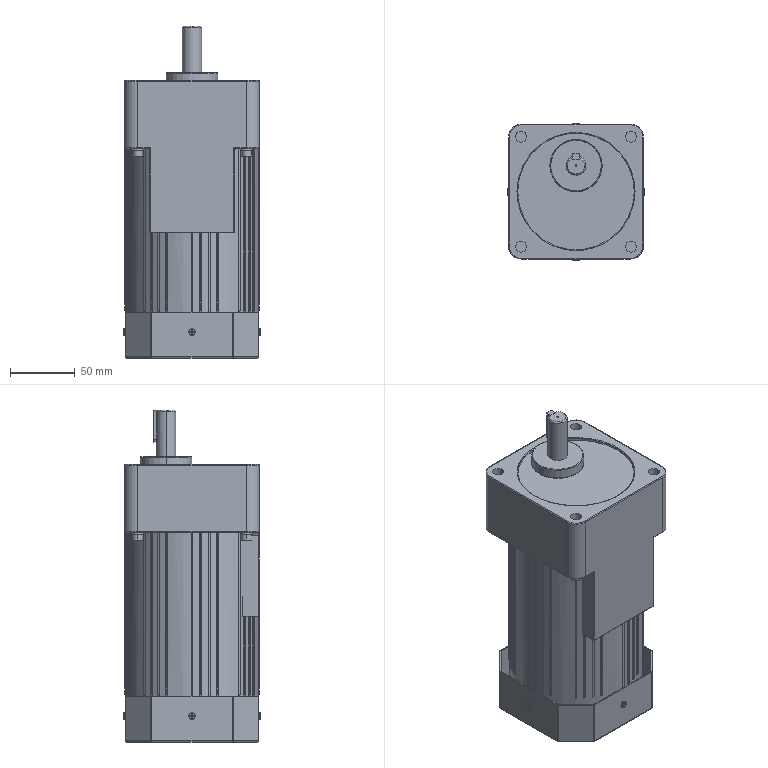Part | SolidWorks | features BaseBody 1 | 1 solid | 514 faces | box 105 x 105 x 256 mm | volume 1923249 mm3 | plane 275 | cylinder 180 | spline 54 | cone 5 | commonest cylinder face diameters 0.4 x102 2 x16 1 x15 5 x9 7.8 x8 8.5 x8